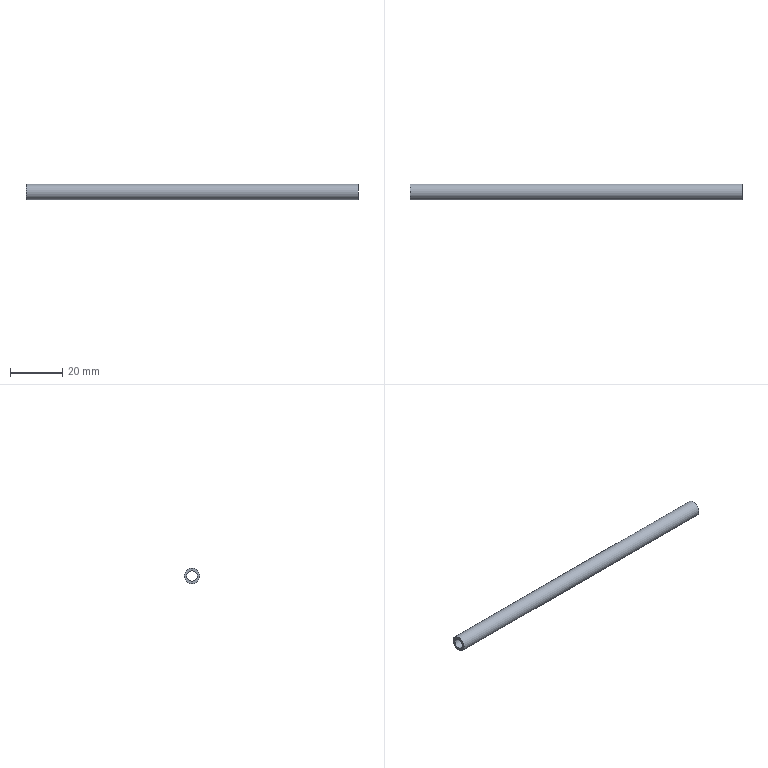Part | NX | features solid 2 | 1 solid | 4 faces | box 127.125 x 6 x 6 mm | volume 1997 mm3 | cylinder 2 | plane 2 | commonest cylinder face diameters 4 x1 6 x1
STEP:
#1=CARTESIAN_POINT('',(257.125,45.,347.));
#2=VERTEX_POINT('',#1);
#3=CARTESIAN_POINT('',(257.125,47.,347.));
#4=DIRECTION('',(-1.,0.,0.));
#5=DIRECTION('',(0.,-1.,0.));
#6=AXIS2_PLACEMENT_3D('',#3,#4,#5);
#7=CIRCLE('',#6,2.);
#8=EDGE_CURVE('',#2,#2,#7,.T.);
#9=ORIENTED_EDGE('',*,*,#8,.F.);
#10=EDGE_LOOP('',(#9));
#11=FACE_BOUND('',#10,.T.);
#12=CARTESIAN_POINT('',(130.,45.,347.));
#13=VERTEX_POINT('',#12);
#14=CARTESIAN_POINT('',(130.,47.,347.));
#15=DIRECTION('',(-1.,0.,0.));
#16=DIRECTION('',(0.,-1.,0.));
#17=AXIS2_PLACEMENT_3D('',#14,#15,#16);
#18=CIRCLE('',#17,2.);
#19=EDGE_CURVE('',#13,#13,#18,.T.);
#20=ORIENTED_EDGE('',*,*,#19,.T.);
#21=EDGE_LOOP('',(#20));
#22=FACE_BOUND('',#21,.T.);
#23=CARTESIAN_POINT('',(216.176,47.,347.));
#24=DIRECTION('',(1.,0.,0.));
#25=DIRECTION('',(0.,1.,0.));
#26=AXIS2_PLACEMENT_3D('',#23,#24,#25);
#27=CYLINDRICAL_SURFACE('',#26,2.);
#28=ADVANCED_FACE('',(#11,#22),#27,.F.);
#29=CARTESIAN_POINT('',(257.125,44.,347.));
#30=VERTEX_POINT('',#29);
#31=CARTESIAN_POINT('',(257.125,47.,347.));
#32=DIRECTION('',(-1.,0.,0.));
#33=DIRECTION('',(0.,-1.,0.));
#34=AXIS2_PLACEMENT_3D('',#31,#32,#33);
#35=CIRCLE('',#34,3.);
#36=EDGE_CURVE('',#30,#30,#35,.T.);
#37=ORIENTED_EDGE('',*,*,#36,.T.);
#38=EDGE_LOOP('',(#37));
#39=FACE_BOUND('',#38,.T.);
#40=CARTESIAN_POINT('',(130.,44.,347.));
#41=VERTEX_POINT('',#40);
#42=CARTESIAN_POINT('',(130.,47.,347.));
#43=DIRECTION('',(-1.,0.,0.));
#44=DIRECTION('',(0.,-1.,0.));
#45=AXIS2_PLACEMENT_3D('',#42,#43,#44);
#46=CIRCLE('',#45,3.);
#47=EDGE_CURVE('',#41,#41,#46,.T.);
#48=ORIENTED_EDGE('',*,*,#47,.F.);
#49=EDGE_LOOP('',(#48));
#50=FACE_BOUND('',#49,.T.);
#51=CARTESIAN_POINT('',(216.176,47.,347.));
#52=DIRECTION('',(1.,0.,0.));
#53=DIRECTION('',(0.,1.,0.));
#54=AXIS2_PLACEMENT_3D('',#51,#52,#53);
#55=CYLINDRICAL_SURFACE('',#54,3.);
#56=ADVANCED_FACE('',(#39,#50),#55,.T.);
#57=ORIENTED_EDGE('',*,*,#8,.T.);
#58=EDGE_LOOP('',(#57));
#59=FACE_BOUND('',#58,.T.);
#60=ORIENTED_EDGE('',*,*,#36,.F.);
#61=EDGE_LOOP('',(#60));
#62=FACE_BOUND('',#61,.T.);
#63=CARTESIAN_POINT('',(257.125,92.83,185.));
#64=DIRECTION('',(-1.,0.,0.));
#65=DIRECTION('',(0.,-1.,0.));
#66=AXIS2_PLACEMENT_3D('',#63,#64,#65);
#67=PLANE('',#66);
#68=ADVANCED_FACE('',(#59,#62),#67,.F.);
#69=ORIENTED_EDGE('',*,*,#19,.F.);
#70=EDGE_LOOP('',(#69));
#71=FACE_BOUND('',#70,.T.);
#72=ORIENTED_EDGE('',*,*,#47,.T.);
#73=EDGE_LOOP('',(#72));
#74=FACE_BOUND('',#73,.T.);
#75=CARTESIAN_POINT('',(130.,35.,347.));
#76=DIRECTION('',(-1.,0.,0.));
#77=DIRECTION('',(0.,-1.,0.));
#78=AXIS2_PLACEMENT_3D('',#75,#76,#77);
#79=PLANE('',#78);
#80=ADVANCED_FACE('',(#71,#74),#79,.T.);
#81=CLOSED_SHELL('',(#28,#56,#68,#80));
#82=MANIFOLD_SOLID_BREP('',#81);
#83=(LENGTH_UNIT()NAMED_UNIT(*)SI_UNIT(.MILLI.,.METRE.));
#84=UNCERTAINTY_MEASURE_WITH_UNIT(LENGTH_MEASURE(0.00001),#83,'','');
#85=(NAMED_UNIT(*)PLANE_ANGLE_UNIT()SI_UNIT($,.RADIAN.));
#86=(NAMED_UNIT(*)SI_UNIT($,.STERADIAN.)SOLID_ANGLE_UNIT());
#87=(GEOMETRIC_REPRESENTATION_CONTEXT(3)GLOBAL_UNCERTAINTY_ASSIGNED_CONTEXT((#84))GLOBAL_UNIT_ASSIGNED_CONTEXT((#83,#85,#86))REPRESENTATION_CONTEXT('',''));
#88=ADVANCED_BREP_SHAPE_REPRESENTATION('',(#82),#87);